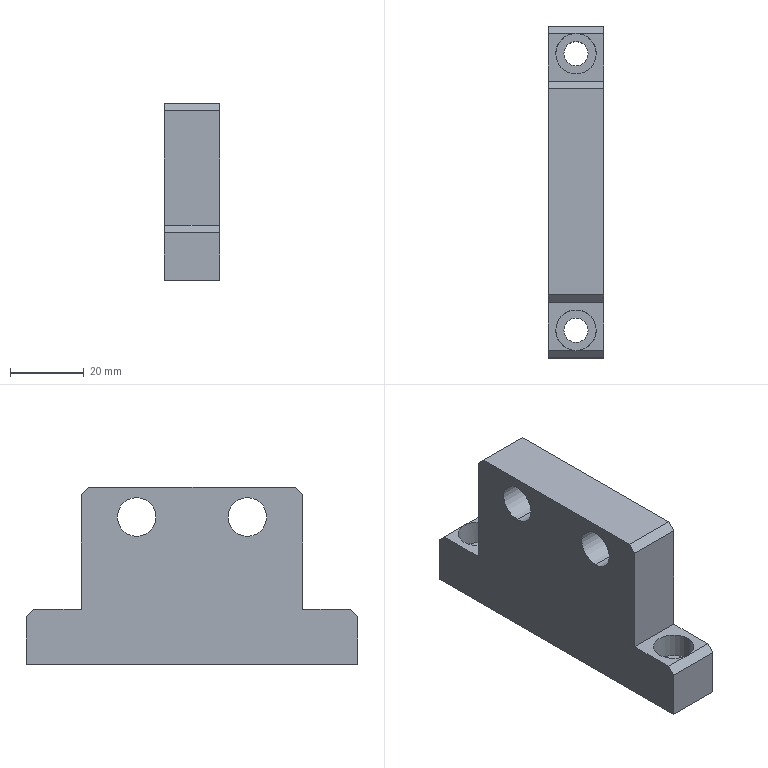Part | SolidWorks | features HoleWzd 2, Chamfer 1, Cut 1, Extrusion 1, MirrorPattern 1 | 1 solid | 28 faces | box 15 x 90 x 48 mm | volume 45379 mm3 | plane 16 | cylinder 12 | commonest cylinder face diameters 6.6 x4 10.5 x4 11 x4
STEP:
#1=CARTESIAN_POINT('',(-7.5,-15.,21.25));
#2=VERTEX_POINT('',#1);
#3=CARTESIAN_POINT('',(-7.5,-15.,10.75));
#4=VERTEX_POINT('',#3);
#5=CARTESIAN_POINT('',(-7.5,-15.,16.));
#6=DIRECTION('',(1.,0.,0.));
#7=DIRECTION('',(0.,0.,-1.));
#8=AXIS2_PLACEMENT_3D('',#5,#6,#7);
#9=CIRCLE('',#8,5.25);
#10=EDGE_CURVE('',#2,#4,#9,.T.);
#11=ORIENTED_EDGE('',*,*,#10,.F.);
#12=CARTESIAN_POINT('',(7.5,-15.,21.25));
#13=VERTEX_POINT('',#12);
#14=CARTESIAN_POINT('',(7.5,-15.,21.25));
#15=DIRECTION('',(1.,0.,0.));
#16=VECTOR('',#15,1000.);
#17=LINE('',#14,#16);
#18=EDGE_CURVE('',#2,#13,#17,.T.);
#19=ORIENTED_EDGE('',*,*,#18,.T.);
#20=CARTESIAN_POINT('',(7.5,-15.,10.75));
#21=VERTEX_POINT('',#20);
#22=CARTESIAN_POINT('',(7.5,-15.,16.));
#23=DIRECTION('',(1.,0.,0.));
#24=DIRECTION('',(0.,0.,-1.));
#25=AXIS2_PLACEMENT_3D('',#22,#23,#24);
#26=CIRCLE('',#25,5.25);
#27=EDGE_CURVE('',#13,#21,#26,.T.);
#28=ORIENTED_EDGE('',*,*,#27,.T.);
#29=CARTESIAN_POINT('',(7.5,-15.,10.75));
#30=DIRECTION('',(1.,0.,0.));
#31=VECTOR('',#30,1000.);
#32=LINE('',#29,#31);
#33=EDGE_CURVE('',#4,#21,#32,.T.);
#34=ORIENTED_EDGE('',*,*,#33,.F.);
#35=EDGE_LOOP('',(#11,#19,#28,#34));
#36=FACE_OUTER_BOUND('',#35,.T.);
#37=CARTESIAN_POINT('',(7.5,-15.,16.));
#38=DIRECTION('',(1.,0.,0.));
#39=DIRECTION('',(0.,0.,-1.));
#40=AXIS2_PLACEMENT_3D('',#37,#38,#39);
#41=CYLINDRICAL_SURFACE('',#40,5.25);
#42=ADVANCED_FACE('',(#36),#41,.F.);
#43=CARTESIAN_POINT('',(-7.5,15.,21.25));
#44=VERTEX_POINT('',#43);
#45=CARTESIAN_POINT('',(-7.5,15.,10.75));
#46=VERTEX_POINT('',#45);
#47=CARTESIAN_POINT('',(-7.5,15.,16.));
#48=DIRECTION('',(1.,0.,0.));
#49=DIRECTION('',(0.,0.,-1.));
#50=AXIS2_PLACEMENT_3D('',#47,#48,#49);
#51=CIRCLE('',#50,5.25);
#52=EDGE_CURVE('',#44,#46,#51,.T.);
#53=ORIENTED_EDGE('',*,*,#52,.F.);
#54=CARTESIAN_POINT('',(7.5,15.,21.25));
#55=VERTEX_POINT('',#54);
#56=CARTESIAN_POINT('',(7.5,15.,21.25));
#57=DIRECTION('',(1.,0.,0.));
#58=VECTOR('',#57,1000.);
#59=LINE('',#56,#58);
#60=EDGE_CURVE('',#44,#55,#59,.T.);
#61=ORIENTED_EDGE('',*,*,#60,.T.);
#62=CARTESIAN_POINT('',(7.5,15.,10.75));
#63=VERTEX_POINT('',#62);
#64=CARTESIAN_POINT('',(7.5,15.,16.));
#65=DIRECTION('',(1.,0.,0.));
#66=DIRECTION('',(0.,0.,-1.));
#67=AXIS2_PLACEMENT_3D('',#64,#65,#66);
#68=CIRCLE('',#67,5.25);
#69=EDGE_CURVE('',#55,#63,#68,.T.);
#70=ORIENTED_EDGE('',*,*,#69,.T.);
#71=CARTESIAN_POINT('',(7.5,15.,10.75));
#72=DIRECTION('',(1.,0.,0.));
#73=VECTOR('',#72,1000.);
#74=LINE('',#71,#73);
#75=EDGE_CURVE('',#46,#63,#74,.T.);
#76=ORIENTED_EDGE('',*,*,#75,.F.);
#77=EDGE_LOOP('',(#53,#61,#70,#76));
#78=FACE_OUTER_BOUND('',#77,.T.);
#79=CARTESIAN_POINT('',(7.5,15.,16.));
#80=DIRECTION('',(1.,0.,0.));
#81=DIRECTION('',(0.,0.,-1.));
#82=AXIS2_PLACEMENT_3D('',#79,#80,#81);
#83=CYLINDRICAL_SURFACE('',#82,5.25);
#84=ADVANCED_FACE('',(#78),#83,.F.);
#85=CARTESIAN_POINT('',(-5.5,-37.5,-15.8));
#86=VERTEX_POINT('',#85);
#87=CARTESIAN_POINT('',(5.5,-37.5,-15.8));
#88=VERTEX_POINT('',#87);
#89=CARTESIAN_POINT('',(0.,-37.5,-15.8));
#90=DIRECTION('',(0.,0.,1.));
#91=DIRECTION('',(1.,0.,0.));
#92=AXIS2_PLACEMENT_3D('',#89,#90,#91);
#93=CIRCLE('',#92,5.5);
#94=EDGE_CURVE('',#86,#88,#93,.T.);
#95=ORIENTED_EDGE('',*,*,#94,.F.);
#96=CARTESIAN_POINT('',(-5.5,-37.5,-9.));
#97=VERTEX_POINT('',#96);
#98=CARTESIAN_POINT('',(-5.5,-37.5,-9.));
#99=DIRECTION('',(0.,0.,1.));
#100=VECTOR('',#99,1000.);
#101=LINE('',#98,#100);
#102=EDGE_CURVE('',#86,#97,#101,.T.);
#103=ORIENTED_EDGE('',*,*,#102,.T.);
#104=CARTESIAN_POINT('',(0.,-43.,-9.));
#105=VERTEX_POINT('',#104);
#106=CARTESIAN_POINT('',(0.,-37.5,-9.));
#107=DIRECTION('',(0.,0.,1.));
#108=DIRECTION('',(1.,0.,0.));
#109=AXIS2_PLACEMENT_3D('',#106,#107,#108);
#110=CIRCLE('',#109,5.5);
#111=EDGE_CURVE('',#97,#105,#110,.T.);
#112=ORIENTED_EDGE('',*,*,#111,.T.);
#113=CARTESIAN_POINT('',(5.5,-37.5,-9.));
#114=VERTEX_POINT('',#113);
#115=CARTESIAN_POINT('',(0.,-37.5,-9.));
#116=DIRECTION('',(0.,0.,1.));
#117=DIRECTION('',(1.,0.,0.));
#118=AXIS2_PLACEMENT_3D('',#115,#116,#117);
#119=CIRCLE('',#118,5.5);
#120=EDGE_CURVE('',#105,#114,#119,.T.);
#121=ORIENTED_EDGE('',*,*,#120,.T.);
#122=CARTESIAN_POINT('',(5.5,-37.5,-9.));
#123=DIRECTION('',(0.,0.,1.));
#124=VECTOR('',#123,1000.);
#125=LINE('',#122,#124);
#126=EDGE_CURVE('',#88,#114,#125,.T.);
#127=ORIENTED_EDGE('',*,*,#126,.F.);
#128=EDGE_LOOP('',(#95,#103,#112,#121,#127));
#129=FACE_OUTER_BOUND('',#128,.T.);
#130=CARTESIAN_POINT('',(0.,-37.5,-9.));
#131=DIRECTION('',(0.,0.,1.));
#132=DIRECTION('',(1.,0.,0.));
#133=AXIS2_PLACEMENT_3D('',#130,#131,#132);
#134=CYLINDRICAL_SURFACE('',#133,5.5);
#135=ADVANCED_FACE('',(#129),#134,.F.);
#136=CARTESIAN_POINT('',(-3.3,-37.5,-24.));
#137=VERTEX_POINT('',#136);
#138=CARTESIAN_POINT('',(3.3,-37.5,-24.));
#139=VERTEX_POINT('',#138);
#140=CARTESIAN_POINT('',(0.,-37.5,-24.));
#141=DIRECTION('',(0.,0.,1.));
#142=DIRECTION('',(1.,0.,0.));
#143=AXIS2_PLACEMENT_3D('',#140,#141,#142);
#144=CIRCLE('',#143,3.3);
#145=EDGE_CURVE('',#137,#139,#144,.T.);
#146=ORIENTED_EDGE('',*,*,#145,.F.);
#147=CARTESIAN_POINT('',(-3.3,-37.5,-15.8));
#148=VERTEX_POINT('',#147);
#149=CARTESIAN_POINT('',(-3.3,-37.5,-9.));
#150=DIRECTION('',(0.,0.,1.));
#151=VECTOR('',#150,1000.);
#152=LINE('',#149,#151);
#153=EDGE_CURVE('',#137,#148,#152,.T.);
#154=ORIENTED_EDGE('',*,*,#153,.T.);
#155=CARTESIAN_POINT('',(3.3,-37.5,-15.8));
#156=VERTEX_POINT('',#155);
#157=CARTESIAN_POINT('',(0.,-37.5,-15.8));
#158=DIRECTION('',(0.,0.,1.));
#159=DIRECTION('',(1.,0.,0.));
#160=AXIS2_PLACEMENT_3D('',#157,#158,#159);
#161=CIRCLE('',#160,3.3);
#162=EDGE_CURVE('',#148,#156,#161,.T.);
#163=ORIENTED_EDGE('',*,*,#162,.T.);
#164=CARTESIAN_POINT('',(3.3,-37.5,-9.));
#165=DIRECTION('',(0.,0.,1.));
#166=VECTOR('',#165,1000.);
#167=LINE('',#164,#166);
#168=EDGE_CURVE('',#139,#156,#167,.T.);
#169=ORIENTED_EDGE('',*,*,#168,.F.);
#170=EDGE_LOOP('',(#146,#154,#163,#169));
#171=FACE_OUTER_BOUND('',#170,.T.);
#172=CARTESIAN_POINT('',(0.,-37.5,-9.));
#173=DIRECTION('',(0.,0.,1.));
#174=DIRECTION('',(1.,0.,0.));
#175=AXIS2_PLACEMENT_3D('',#172,#173,#174);
#176=CYLINDRICAL_SURFACE('',#175,3.3);
#177=ADVANCED_FACE('',(#171),#176,.F.);
#178=CARTESIAN_POINT('',(-5.5,37.5,-15.8));
#179=VERTEX_POINT('',#178);
#180=CARTESIAN_POINT('',(5.5,37.5,-15.8));
#181=VERTEX_POINT('',#180);
#182=CARTESIAN_POINT('',(0.,37.5,-15.8));
#183=DIRECTION('',(0.,0.,1.));
#184=DIRECTION('',(1.,0.,0.));
#185=AXIS2_PLACEMENT_3D('',#182,#183,#184);
#186=CIRCLE('',#185,5.5);
#187=EDGE_CURVE('',#179,#181,#186,.T.);
#188=ORIENTED_EDGE('',*,*,#187,.F.);
#189=CARTESIAN_POINT('',(-5.5,37.5,-9.));
#190=VERTEX_POINT('',#189);
#191=CARTESIAN_POINT('',(-5.5,37.5,-9.));
#192=DIRECTION('',(0.,0.,1.));
#193=VECTOR('',#192,1000.);
#194=LINE('',#191,#193);
#195=EDGE_CURVE('',#179,#190,#194,.T.);
#196=ORIENTED_EDGE('',*,*,#195,.T.);
#197=CARTESIAN_POINT('',(5.5,37.5,-9.));
#198=VERTEX_POINT('',#197);
#199=CARTESIAN_POINT('',(0.,37.5,-9.));
#200=DIRECTION('',(0.,0.,1.));
#201=DIRECTION('',(1.,0.,0.));
#202=AXIS2_PLACEMENT_3D('',#199,#200,#201);
#203=CIRCLE('',#202,5.5);
#204=EDGE_CURVE('',#190,#198,#203,.T.);
#205=ORIENTED_EDGE('',*,*,#204,.T.);
#206=CARTESIAN_POINT('',(5.5,37.5,-9.));
#207=DIRECTION('',(0.,0.,1.));
#208=VECTOR('',#207,1000.);
#209=LINE('',#206,#208);
#210=EDGE_CURVE('',#181,#198,#209,.T.);
#211=ORIENTED_EDGE('',*,*,#210,.F.);
#212=EDGE_LOOP('',(#188,#196,#205,#211));
#213=FACE_OUTER_BOUND('',#212,.T.);
#214=CARTESIAN_POINT('',(0.,37.5,-9.));
#215=DIRECTION('',(0.,0.,1.));
#216=DIRECTION('',(1.,0.,0.));
#217=AXIS2_PLACEMENT_3D('',#214,#215,#216);
#218=CYLINDRICAL_SURFACE('',#217,5.5);
#219=ADVANCED_FACE('',(#213),#218,.F.);
#220=CARTESIAN_POINT('',(-3.3,37.5,-24.));
#221=VERTEX_POINT('',#220);
#222=CARTESIAN_POINT('',(3.3,37.5,-24.));
#223=VERTEX_POINT('',#222);
#224=CARTESIAN_POINT('',(0.,37.5,-24.));
#225=DIRECTION('',(0.,0.,1.));
#226=DIRECTION('',(1.,0.,0.));
#227=AXIS2_PLACEMENT_3D('',#224,#225,#226);
#228=CIRCLE('',#227,3.3);
#229=EDGE_CURVE('',#221,#223,#228,.T.);
#230=ORIENTED_EDGE('',*,*,#229,.F.);
#231=CARTESIAN_POINT('',(-3.3,37.5,-15.8));
#232=VERTEX_POINT('',#231);
#233=CARTESIAN_POINT('',(-3.3,37.5,-9.));
#234=DIRECTION('',(0.,0.,1.));
#235=VECTOR('',#234,1000.);
#236=LINE('',#233,#235);
#237=EDGE_CURVE('',#221,#232,#236,.T.);
#238=ORIENTED_EDGE('',*,*,#237,.T.);
#239=CARTESIAN_POINT('',(3.3,37.5,-15.8));
#240=VERTEX_POINT('',#239);
#241=CARTESIAN_POINT('',(0.,37.5,-15.8));
#242=DIRECTION('',(0.,0.,1.));
#243=DIRECTION('',(1.,0.,0.));
#244=AXIS2_PLACEMENT_3D('',#241,#242,#243);
#245=CIRCLE('',#244,3.3);
#246=EDGE_CURVE('',#232,#240,#245,.T.);
#247=ORIENTED_EDGE('',*,*,#246,.T.);
#248=CARTESIAN_POINT('',(3.3,37.5,-9.));
#249=DIRECTION('',(0.,0.,1.));
#250=VECTOR('',#249,1000.);
#251=LINE('',#248,#250);
#252=EDGE_CURVE('',#223,#240,#251,.T.);
#253=ORIENTED_EDGE('',*,*,#252,.F.);
#254=EDGE_LOOP('',(#230,#238,#247,#253));
#255=FACE_OUTER_BOUND('',#254,.T.);
#256=CARTESIAN_POINT('',(0.,37.5,-9.));
#257=DIRECTION('',(0.,0.,1.));
#258=DIRECTION('',(1.,0.,0.));
#259=AXIS2_PLACEMENT_3D('',#256,#257,#258);
#260=CYLINDRICAL_SURFACE('',#259,3.3);
#261=ADVANCED_FACE('',(#255),#260,.F.);
#262=CARTESIAN_POINT('',(-7.5,-15.,16.));
#263=DIRECTION('',(1.,0.,0.));
#264=DIRECTION('',(0.,0.,-1.));
#265=AXIS2_PLACEMENT_3D('',#262,#263,#264);
#266=CIRCLE('',#265,5.25);
#267=EDGE_CURVE('',#4,#2,#266,.T.);
#268=ORIENTED_EDGE('',*,*,#267,.T.);
#269=ORIENTED_EDGE('',*,*,#10,.T.);
#270=EDGE_LOOP('',(#268,#269));
#271=FACE_BOUND('',#270,.T.);
#272=CARTESIAN_POINT('',(-7.5,15.,16.));
#273=DIRECTION('',(1.,0.,0.));
#274=DIRECTION('',(0.,0.,-1.));
#275=AXIS2_PLACEMENT_3D('',#272,#273,#274);
#276=CIRCLE('',#275,5.25);
#277=EDGE_CURVE('',#46,#44,#276,.T.);
#278=ORIENTED_EDGE('',*,*,#277,.T.);
#279=ORIENTED_EDGE('',*,*,#52,.T.);
#280=EDGE_LOOP('',(#278,#279));
#281=FACE_BOUND('',#280,.T.);
#282=CARTESIAN_POINT('',(-7.5,43.,-9.));
#283=VERTEX_POINT('',#282);
#284=CARTESIAN_POINT('',(-7.5,30.,-9.));
#285=VERTEX_POINT('',#284);
#286=CARTESIAN_POINT('',(-7.5,45.,-9.));
#287=DIRECTION('',(0.,-1.,0.));
#288=VECTOR('',#287,1000.);
#289=LINE('',#286,#288);
#290=EDGE_CURVE('',#283,#285,#289,.T.);
#291=ORIENTED_EDGE('',*,*,#290,.F.);
#292=CARTESIAN_POINT('',(-7.5,45.,-11.));
#293=VERTEX_POINT('',#292);
#294=CARTESIAN_POINT('',(-7.5,45.,-11.));
#295=DIRECTION('',(0.,0.7071,-0.7071));
#296=VECTOR('',#295,1000.);
#297=LINE('',#294,#296);
#298=EDGE_CURVE('',#283,#293,#297,.T.);
#299=ORIENTED_EDGE('',*,*,#298,.T.);
#300=CARTESIAN_POINT('',(-7.5,45.,-24.));
#301=VERTEX_POINT('',#300);
#302=CARTESIAN_POINT('',(-7.5,45.,24.));
#303=DIRECTION('',(0.,0.,1.));
#304=VECTOR('',#303,1000.);
#305=LINE('',#302,#304);
#306=EDGE_CURVE('',#301,#293,#305,.T.);
#307=ORIENTED_EDGE('',*,*,#306,.F.);
#308=CARTESIAN_POINT('',(-7.5,-45.,-24.));
#309=VERTEX_POINT('',#308);
#310=CARTESIAN_POINT('',(-7.5,45.,-24.));
#311=DIRECTION('',(0.,-1.,0.));
#312=VECTOR('',#311,1000.);
#313=LINE('',#310,#312);
#314=EDGE_CURVE('',#301,#309,#313,.T.);
#315=ORIENTED_EDGE('',*,*,#314,.T.);
#316=CARTESIAN_POINT('',(-7.5,-45.,-11.));
#317=VERTEX_POINT('',#316);
#318=CARTESIAN_POINT('',(-7.5,-45.,24.));
#319=DIRECTION('',(0.,0.,1.));
#320=VECTOR('',#319,1000.);
#321=LINE('',#318,#320);
#322=EDGE_CURVE('',#309,#317,#321,.T.);
#323=ORIENTED_EDGE('',*,*,#322,.T.);
#324=CARTESIAN_POINT('',(-7.5,-43.,-9.));
#325=VERTEX_POINT('',#324);
#326=CARTESIAN_POINT('',(-7.5,-43.,-9.));
#327=DIRECTION('',(0.,0.7071,0.7071));
#328=VECTOR('',#327,1000.);
#329=LINE('',#326,#328);
#330=EDGE_CURVE('',#317,#325,#329,.T.);
#331=ORIENTED_EDGE('',*,*,#330,.T.);
#332=CARTESIAN_POINT('',(-7.5,-30.,-9.));
#333=VERTEX_POINT('',#332);
#334=CARTESIAN_POINT('',(-7.5,-45.,-9.));
#335=DIRECTION('',(0.,1.,0.));
#336=VECTOR('',#335,1000.);
#337=LINE('',#334,#336);
#338=EDGE_CURVE('',#325,#333,#337,.T.);
#339=ORIENTED_EDGE('',*,*,#338,.T.);
#340=CARTESIAN_POINT('',(-7.5,-30.,22.));
#341=VERTEX_POINT('',#340);
#342=CARTESIAN_POINT('',(-7.5,-30.,24.));
#343=DIRECTION('',(0.,0.,1.));
#344=VECTOR('',#343,1000.);
#345=LINE('',#342,#344);
#346=EDGE_CURVE('',#333,#341,#345,.T.);
#347=ORIENTED_EDGE('',*,*,#346,.T.);
#348=CARTESIAN_POINT('',(-7.5,-28.,24.));
#349=VERTEX_POINT('',#348);
#350=CARTESIAN_POINT('',(-7.5,-28.,24.));
#351=DIRECTION('',(0.,0.7071,0.7071));
#352=VECTOR('',#351,1000.);
#353=LINE('',#350,#352);
#354=EDGE_CURVE('',#341,#349,#353,.T.);
#355=ORIENTED_EDGE('',*,*,#354,.T.);
#356=CARTESIAN_POINT('',(-7.5,28.,24.));
#357=VERTEX_POINT('',#356);
#358=CARTESIAN_POINT('',(-7.5,45.,24.));
#359=DIRECTION('',(0.,-1.,0.));
#360=VECTOR('',#359,1000.);
#361=LINE('',#358,#360);
#362=EDGE_CURVE('',#357,#349,#361,.T.);
#363=ORIENTED_EDGE('',*,*,#362,.F.);
#364=CARTESIAN_POINT('',(-7.5,30.,22.));
#365=VERTEX_POINT('',#364);
#366=CARTESIAN_POINT('',(-7.5,30.,22.));
#367=DIRECTION('',(0.,0.7071,-0.7071));
#368=VECTOR('',#367,1000.);
#369=LINE('',#366,#368);
#370=EDGE_CURVE('',#357,#365,#369,.T.);
#371=ORIENTED_EDGE('',*,*,#370,.T.);
#372=CARTESIAN_POINT('',(-7.5,30.,24.));
#373=DIRECTION('',(0.,0.,1.));
#374=VECTOR('',#373,1000.);
#375=LINE('',#372,#374);
#376=EDGE_CURVE('',#285,#365,#375,.T.);
#377=ORIENTED_EDGE('',*,*,#376,.F.);
#378=EDGE_LOOP('',(#291,#299,#307,#315,#323,#331,#339,#347,#355,#363,#371,#377));
#379=FACE_OUTER_BOUND('',#378,.T.);
#380=CARTESIAN_POINT('',(-7.5,45.,24.));
#381=DIRECTION('',(1.,0.,0.));
#382=DIRECTION('',(0.,0.,-1.));
#383=AXIS2_PLACEMENT_3D('',#380,#381,#382);
#384=PLANE('',#383);
#385=ADVANCED_FACE('',(#271,#281,#379),#384,.F.);
#386=ORIENTED_EDGE('',*,*,#362,.T.);
#387=CARTESIAN_POINT('',(7.5,-28.,24.));
#388=VERTEX_POINT('',#387);
#389=CARTESIAN_POINT('',(7.5,-28.,24.));
#390=DIRECTION('',(1.,0.,0.));
#391=VECTOR('',#390,1000.);
#392=LINE('',#389,#391);
#393=EDGE_CURVE('',#349,#388,#392,.T.);
#394=ORIENTED_EDGE('',*,*,#393,.T.);
#395=CARTESIAN_POINT('',(7.5,28.,24.));
#396=VERTEX_POINT('',#395);
#397=CARTESIAN_POINT('',(7.5,45.,24.));
#398=DIRECTION('',(0.,-1.,0.));
#399=VECTOR('',#398,1000.);
#400=LINE('',#397,#399);
#401=EDGE_CURVE('',#396,#388,#400,.T.);
#402=ORIENTED_EDGE('',*,*,#401,.F.);
#403=CARTESIAN_POINT('',(-7.5,28.,24.));
#404=DIRECTION('',(-1.,0.,0.));
#405=VECTOR('',#404,1000.);
#406=LINE('',#403,#405);
#407=EDGE_CURVE('',#396,#357,#406,.T.);
#408=ORIENTED_EDGE('',*,*,#407,.T.);
#409=EDGE_LOOP('',(#386,#394,#402,#408));
#410=FACE_OUTER_BOUND('',#409,.T.);
#411=CARTESIAN_POINT('',(7.5,45.,24.));
#412=DIRECTION('',(0.,0.,-1.));
#413=DIRECTION('',(-1.,0.,0.));
#414=AXIS2_PLACEMENT_3D('',#411,#412,#413);
#415=PLANE('',#414);
#416=ADVANCED_FACE('',(#410),#415,.F.);
#417=CARTESIAN_POINT('',(7.5,-15.,16.));
#418=DIRECTION('',(1.,0.,0.));
#419=DIRECTION('',(0.,0.,-1.));
#420=AXIS2_PLACEMENT_3D('',#417,#418,#419);
#421=CIRCLE('',#420,5.25);
#422=EDGE_CURVE('',#21,#13,#421,.T.);
#423=ORIENTED_EDGE('',*,*,#422,.F.);
#424=ORIENTED_EDGE('',*,*,#27,.F.);
#425=EDGE_LOOP('',(#423,#424));
#426=FACE_BOUND('',#425,.T.);
#427=CARTESIAN_POINT('',(7.5,15.,16.));
#428=DIRECTION('',(1.,0.,0.));
#429=DIRECTION('',(0.,0.,-1.));
#430=AXIS2_PLACEMENT_3D('',#427,#428,#429);
#431=CIRCLE('',#430,5.25);
#432=EDGE_CURVE('',#63,#55,#431,.T.);
#433=ORIENTED_EDGE('',*,*,#432,.F.);
#434=ORIENTED_EDGE('',*,*,#69,.F.);
#435=EDGE_LOOP('',(#433,#434));
#436=FACE_BOUND('',#435,.T.);
#437=CARTESIAN_POINT('',(7.5,45.,-11.));
#438=VERTEX_POINT('',#437);
#439=CARTESIAN_POINT('',(7.5,45.,-24.));
#440=VERTEX_POINT('',#439);
#441=CARTESIAN_POINT('',(7.5,45.,24.));
#442=DIRECTION('',(0.,0.,-1.));
#443=VECTOR('',#442,1000.);
#444=LINE('',#441,#443);
#445=EDGE_CURVE('',#438,#440,#444,.T.);
#446=ORIENTED_EDGE('',*,*,#445,.F.);
#447=CARTESIAN_POINT('',(7.5,43.,-9.));
#448=VERTEX_POINT('',#447);
#449=CARTESIAN_POINT('',(7.5,45.,-11.));
#450=DIRECTION('',(0.,-0.7071,0.7071));
#451=VECTOR('',#450,1000.);
#452=LINE('',#449,#451);
#453=EDGE_CURVE('',#438,#448,#452,.T.);
#454=ORIENTED_EDGE('',*,*,#453,.T.);
#455=CARTESIAN_POINT('',(7.5,30.,-9.));
#456=VERTEX_POINT('',#455);
#457=CARTESIAN_POINT('',(7.5,45.,-9.));
#458=DIRECTION('',(0.,-1.,0.));
#459=VECTOR('',#458,1000.);
#460=LINE('',#457,#459);
#461=EDGE_CURVE('',#448,#456,#460,.T.);
#462=ORIENTED_EDGE('',*,*,#461,.T.);
#463=CARTESIAN_POINT('',(7.5,30.,22.));
#464=VERTEX_POINT('',#463);
#465=CARTESIAN_POINT('',(7.5,30.,24.));
#466=DIRECTION('',(0.,0.,1.));
#467=VECTOR('',#466,1000.);
#468=LINE('',#465,#467);
#469=EDGE_CURVE('',#456,#464,#468,.T.);
#470=ORIENTED_EDGE('',*,*,#469,.T.);
#471=CARTESIAN_POINT('',(7.5,30.,22.));
#472=DIRECTION('',(0.,-0.7071,0.7071));
#473=VECTOR('',#472,1000.);
#474=LINE('',#471,#473);
#475=EDGE_CURVE('',#464,#396,#474,.T.);
#476=ORIENTED_EDGE('',*,*,#475,.T.);
#477=ORIENTED_EDGE('',*,*,#401,.T.);
#478=CARTESIAN_POINT('',(7.5,-30.,22.));
#479=VERTEX_POINT('',#478);
#480=CARTESIAN_POINT('',(7.5,-28.,24.));
#481=DIRECTION('',(0.,-0.7071,-0.7071));
#482=VECTOR('',#481,1000.);
#483=LINE('',#480,#482);
#484=EDGE_CURVE('',#388,#479,#483,.T.);
#485=ORIENTED_EDGE('',*,*,#484,.T.);
#486=CARTESIAN_POINT('',(7.5,-30.,-9.));
#487=VERTEX_POINT('',#486);
#488=CARTESIAN_POINT('',(7.5,-30.,24.));
#489=DIRECTION('',(0.,0.,1.));
#490=VECTOR('',#489,1000.);
#491=LINE('',#488,#490);
#492=EDGE_CURVE('',#487,#479,#491,.T.);
#493=ORIENTED_EDGE('',*,*,#492,.F.);
#494=CARTESIAN_POINT('',(7.5,-43.,-9.));
#495=VERTEX_POINT('',#494);
#496=CARTESIAN_POINT('',(7.5,-45.,-9.));
#497=DIRECTION('',(0.,1.,0.));
#498=VECTOR('',#497,1000.);
#499=LINE('',#496,#498);
#500=EDGE_CURVE('',#495,#487,#499,.T.);
#501=ORIENTED_EDGE('',*,*,#500,.F.);
#502=CARTESIAN_POINT('',(7.5,-45.,-11.));
#503=VERTEX_POINT('',#502);
#504=CARTESIAN_POINT('',(7.5,-43.,-9.));
#505=DIRECTION('',(0.,-0.7071,-0.7071));
#506=VECTOR('',#505,1000.);
#507=LINE('',#504,#506);
#508=EDGE_CURVE('',#495,#503,#507,.T.);
#509=ORIENTED_EDGE('',*,*,#508,.T.);
#510=CARTESIAN_POINT('',(7.5,-45.,-24.));
#511=VERTEX_POINT('',#510);
#512=CARTESIAN_POINT('',(7.5,-45.,24.));
#513=DIRECTION('',(0.,0.,-1.));
#514=VECTOR('',#513,1000.);
#515=LINE('',#512,#514);
#516=EDGE_CURVE('',#503,#511,#515,.T.);
#517=ORIENTED_EDGE('',*,*,#516,.T.);
#518=CARTESIAN_POINT('',(7.5,45.,-24.));
#519=DIRECTION('',(0.,-1.,0.));
#520=VECTOR('',#519,1000.);
#521=LINE('',#518,#520);
#522=EDGE_CURVE('',#440,#511,#521,.T.);
#523=ORIENTED_EDGE('',*,*,#522,.F.);
#524=EDGE_LOOP('',(#446,#454,#462,#470,#476,#477,#485,#493,#501,#509,#517,#523));
#525=FACE_OUTER_BOUND('',#524,.T.);
#526=CARTESIAN_POINT('',(7.5,45.,24.));
#527=DIRECTION('',(-1.,0.,0.));
#528=DIRECTION('',(0.,0.,1.));
#529=AXIS2_PLACEMENT_3D('',#526,#527,#528);
#530=PLANE('',#529);
#531=ADVANCED_FACE('',(#426,#436,#525),#530,.F.);
#532=ORIENTED_EDGE('',*,*,#306,.T.);
#533=CARTESIAN_POINT('',(0.,45.,-11.));
#534=DIRECTION('',(1.,0.,0.));
#535=VECTOR('',#534,1000.);
#536=LINE('',#533,#535);
#537=EDGE_CURVE('',#293,#438,#536,.T.);
#538=ORIENTED_EDGE('',*,*,#537,.T.);
#539=ORIENTED_EDGE('',*,*,#445,.T.);
#540=CARTESIAN_POINT('',(7.5,45.,-24.));
#541=DIRECTION('',(-1.,0.,0.));
#542=VECTOR('',#541,1000.);
#543=LINE('',#540,#542);
#544=EDGE_CURVE('',#440,#301,#543,.T.);
#545=ORIENTED_EDGE('',*,*,#544,.T.);
#546=EDGE_LOOP('',(#532,#538,#539,#545));
#547=FACE_OUTER_BOUND('',#546,.T.);
#548=CARTESIAN_POINT('',(0.,45.,0.));
#549=DIRECTION('',(0.,1.,0.));
#550=DIRECTION('',(0.,0.,1.));
#551=AXIS2_PLACEMENT_3D('',#548,#549,#550);
#552=PLANE('',#551);
#553=ADVANCED_FACE('',(#547),#552,.T.);
#554=CARTESIAN_POINT('',(0.,-37.5,-24.));
#555=DIRECTION('',(0.,0.,1.));
#556=DIRECTION('',(1.,0.,0.));
#557=AXIS2_PLACEMENT_3D('',#554,#555,#556);
#558=CIRCLE('',#557,3.3);
#559=EDGE_CURVE('',#139,#137,#558,.T.);
#560=ORIENTED_EDGE('',*,*,#559,.T.);
#561=ORIENTED_EDGE('',*,*,#145,.T.);
#562=EDGE_LOOP('',(#560,#561));
#563=FACE_BOUND('',#562,.T.);
#564=CARTESIAN_POINT('',(0.,37.5,-24.));
#565=DIRECTION('',(0.,0.,1.));
#566=DIRECTION('',(1.,0.,0.));
#567=AXIS2_PLACEMENT_3D('',#564,#565,#566);
#568=CIRCLE('',#567,3.3);
#569=EDGE_CURVE('',#223,#221,#568,.T.);
#570=ORIENTED_EDGE('',*,*,#569,.T.);
#571=ORIENTED_EDGE('',*,*,#229,.T.);
#572=EDGE_LOOP('',(#570,#571));
#573=FACE_BOUND('',#572,.T.);
#574=CARTESIAN_POINT('',(7.5,-45.,-24.));
#575=DIRECTION('',(-1.,0.,0.));
#576=VECTOR('',#575,1000.);
#577=LINE('',#574,#576);
#578=EDGE_CURVE('',#511,#309,#577,.T.);
#579=ORIENTED_EDGE('',*,*,#578,.T.);
#580=ORIENTED_EDGE('',*,*,#314,.F.);
#581=ORIENTED_EDGE('',*,*,#544,.F.);
#582=ORIENTED_EDGE('',*,*,#522,.T.);
#583=EDGE_LOOP('',(#579,#580,#581,#582));
#584=FACE_OUTER_BOUND('',#583,.T.);
#585=CARTESIAN_POINT('',(7.5,45.,-24.));
#586=DIRECTION('',(0.,0.,1.));
#587=DIRECTION('',(1.,0.,0.));
#588=AXIS2_PLACEMENT_3D('',#585,#586,#587);
#589=PLANE('',#588);
#590=ADVANCED_FACE('',(#563,#573,#584),#589,.F.);
#591=ORIENTED_EDGE('',*,*,#516,.F.);
#592=CARTESIAN_POINT('',(0.,-45.,-11.));
#593=DIRECTION('',(-1.,0.,0.));
#594=VECTOR('',#593,1000.);
#595=LINE('',#592,#594);
#596=EDGE_CURVE('',#503,#317,#595,.T.);
#597=ORIENTED_EDGE('',*,*,#596,.T.);
#598=ORIENTED_EDGE('',*,*,#322,.F.);
#599=ORIENTED_EDGE('',*,*,#578,.F.);
#600=EDGE_LOOP('',(#591,#597,#598,#599));
#601=FACE_OUTER_BOUND('',#600,.T.);
#602=CARTESIAN_POINT('',(0.,-45.,0.));
#603=DIRECTION('',(0.,1.,0.));
#604=DIRECTION('',(0.,0.,1.));
#605=AXIS2_PLACEMENT_3D('',#602,#603,#604);
#606=PLANE('',#605);
#607=ADVANCED_FACE('',(#601),#606,.F.);
#608=ORIENTED_EDGE('',*,*,#492,.T.);
#609=CARTESIAN_POINT('',(-7.5,-30.,22.));
#610=DIRECTION('',(-1.,0.,0.));
#611=VECTOR('',#610,1000.);
#612=LINE('',#609,#611);
#613=EDGE_CURVE('',#479,#341,#612,.T.);
#614=ORIENTED_EDGE('',*,*,#613,.T.);
#615=ORIENTED_EDGE('',*,*,#346,.F.);
#616=CARTESIAN_POINT('',(-7.5,-30.,-9.));
#617=DIRECTION('',(1.,0.,0.));
#618=VECTOR('',#617,1000.);
#619=LINE('',#616,#618);
#620=EDGE_CURVE('',#333,#487,#619,.T.);
#621=ORIENTED_EDGE('',*,*,#620,.T.);
#622=EDGE_LOOP('',(#608,#614,#615,#621));
#623=FACE_OUTER_BOUND('',#622,.T.);
#624=CARTESIAN_POINT('',(-7.5,-30.,24.));
#625=DIRECTION('',(0.,1.,0.));
#626=DIRECTION('',(0.,0.,1.));
#627=AXIS2_PLACEMENT_3D('',#624,#625,#626);
#628=PLANE('',#627);
#629=ADVANCED_FACE('',(#623),#628,.F.);
#630=ORIENTED_EDGE('',*,*,#338,.F.);
#631=CARTESIAN_POINT('',(-7.5,-43.,-9.));
#632=DIRECTION('',(1.,0.,0.));
#633=VECTOR('',#632,1000.);
#634=LINE('',#631,#633);
#635=EDGE_CURVE('',#325,#105,#634,.T.);
#636=ORIENTED_EDGE('',*,*,#635,.T.);
#637=ORIENTED_EDGE('',*,*,#111,.F.);
#638=CARTESIAN_POINT('',(0.,-37.5,-9.));
#639=DIRECTION('',(0.,0.,1.));
#640=DIRECTION('',(1.,0.,0.));
#641=AXIS2_PLACEMENT_3D('',#638,#639,#640);
#642=CIRCLE('',#641,5.5);
#643=EDGE_CURVE('',#114,#97,#642,.T.);
#644=ORIENTED_EDGE('',*,*,#643,.F.);
#645=ORIENTED_EDGE('',*,*,#120,.F.);
#646=CARTESIAN_POINT('',(-7.5,-43.,-9.));
#647=DIRECTION('',(1.,0.,0.));
#648=VECTOR('',#647,1000.);
#649=LINE('',#646,#648);
#650=EDGE_CURVE('',#105,#495,#649,.T.);
#651=ORIENTED_EDGE('',*,*,#650,.T.);
#652=ORIENTED_EDGE('',*,*,#500,.T.);
#653=ORIENTED_EDGE('',*,*,#620,.F.);
#654=EDGE_LOOP('',(#630,#636,#637,#644,#645,#651,#652,#653));
#655=FACE_OUTER_BOUND('',#654,.T.);
#656=CARTESIAN_POINT('',(-7.5,-45.,-9.));
#657=DIRECTION('',(0.,0.,-1.));
#658=DIRECTION('',(-1.,0.,0.));
#659=AXIS2_PLACEMENT_3D('',#656,#657,#658);
#660=PLANE('',#659);
#661=ADVANCED_FACE('',(#655),#660,.F.);
#662=ORIENTED_EDGE('',*,*,#461,.F.);
#663=CARTESIAN_POINT('',(0.,43.,-9.));
#664=VERTEX_POINT('',#663);
#665=CARTESIAN_POINT('',(-7.5,43.,-9.));
#666=DIRECTION('',(-1.,0.,0.));
#667=VECTOR('',#666,1000.);
#668=LINE('',#665,#667);
#669=EDGE_CURVE('',#448,#664,#668,.T.);
#670=ORIENTED_EDGE('',*,*,#669,.T.);
#671=CARTESIAN_POINT('',(0.,37.5,-9.));
#672=DIRECTION('',(0.,0.,1.));
#673=DIRECTION('',(1.,0.,0.));
#674=AXIS2_PLACEMENT_3D('',#671,#672,#673);
#675=CIRCLE('',#674,5.5);
#676=EDGE_CURVE('',#198,#664,#675,.T.);
#677=ORIENTED_EDGE('',*,*,#676,.F.);
#678=ORIENTED_EDGE('',*,*,#204,.F.);
#679=CARTESIAN_POINT('',(0.,37.5,-9.));
#680=DIRECTION('',(0.,0.,1.));
#681=DIRECTION('',(1.,0.,0.));
#682=AXIS2_PLACEMENT_3D('',#679,#680,#681);
#683=CIRCLE('',#682,5.5);
#684=EDGE_CURVE('',#664,#190,#683,.T.);
#685=ORIENTED_EDGE('',*,*,#684,.F.);
#686=CARTESIAN_POINT('',(-7.5,43.,-9.));
#687=DIRECTION('',(-1.,0.,0.));
#688=VECTOR('',#687,1000.);
#689=LINE('',#686,#688);
#690=EDGE_CURVE('',#664,#283,#689,.T.);
#691=ORIENTED_EDGE('',*,*,#690,.T.);
#692=ORIENTED_EDGE('',*,*,#290,.T.);
#693=CARTESIAN_POINT('',(-7.5,30.,-9.));
#694=DIRECTION('',(1.,0.,0.));
#695=VECTOR('',#694,1000.);
#696=LINE('',#693,#695);
#697=EDGE_CURVE('',#285,#456,#696,.T.);
#698=ORIENTED_EDGE('',*,*,#697,.T.);
#699=EDGE_LOOP('',(#662,#670,#677,#678,#685,#691,#692,#698));
#700=FACE_OUTER_BOUND('',#699,.T.);
#701=CARTESIAN_POINT('',(-7.5,45.,-9.));
#702=DIRECTION('',(0.,0.,1.));
#703=DIRECTION('',(1.,0.,0.));
#704=AXIS2_PLACEMENT_3D('',#701,#702,#703);
#705=PLANE('',#704);
#706=ADVANCED_FACE('',(#700),#705,.T.);
#707=ORIENTED_EDGE('',*,*,#376,.T.);
#708=CARTESIAN_POINT('',(7.5,30.,22.));
#709=DIRECTION('',(1.,0.,0.));
#710=VECTOR('',#709,1000.);
#711=LINE('',#708,#710);
#712=EDGE_CURVE('',#365,#464,#711,.T.);
#713=ORIENTED_EDGE('',*,*,#712,.T.);
#714=ORIENTED_EDGE('',*,*,#469,.F.);
#715=ORIENTED_EDGE('',*,*,#697,.F.);
#716=EDGE_LOOP('',(#707,#713,#714,#715));
#717=FACE_OUTER_BOUND('',#716,.T.);
#718=CARTESIAN_POINT('',(-7.5,30.,24.));
#719=DIRECTION('',(0.,1.,0.));
#720=DIRECTION('',(0.,0.,1.));
#721=AXIS2_PLACEMENT_3D('',#718,#719,#720);
#722=PLANE('',#721);
#723=ADVANCED_FACE('',(#717),#722,.T.);
#724=ORIENTED_EDGE('',*,*,#237,.F.);
#725=ORIENTED_EDGE('',*,*,#569,.F.);
#726=ORIENTED_EDGE('',*,*,#252,.T.);
#727=CARTESIAN_POINT('',(0.,37.5,-15.8));
#728=DIRECTION('',(0.,0.,1.));
#729=DIRECTION('',(1.,0.,0.));
#730=AXIS2_PLACEMENT_3D('',#727,#728,#729);
#731=CIRCLE('',#730,3.3);
#732=EDGE_CURVE('',#240,#232,#731,.T.);
#733=ORIENTED_EDGE('',*,*,#732,.T.);
#734=EDGE_LOOP('',(#724,#725,#726,#733));
#735=FACE_OUTER_BOUND('',#734,.T.);
#736=CARTESIAN_POINT('',(0.,37.5,-9.));
#737=DIRECTION('',(0.,0.,1.));
#738=DIRECTION('',(1.,0.,0.));
#739=AXIS2_PLACEMENT_3D('',#736,#737,#738);
#740=CYLINDRICAL_SURFACE('',#739,3.3);
#741=ADVANCED_FACE('',(#735),#740,.F.);
#742=ORIENTED_EDGE('',*,*,#732,.F.);
#743=ORIENTED_EDGE('',*,*,#246,.F.);
#744=EDGE_LOOP('',(#742,#743));
#745=FACE_BOUND('',#744,.T.);
#746=CARTESIAN_POINT('',(0.,37.5,-15.8));
#747=DIRECTION('',(0.,0.,1.));
#748=DIRECTION('',(1.,0.,0.));
#749=AXIS2_PLACEMENT_3D('',#746,#747,#748);
#750=CIRCLE('',#749,5.5);
#751=EDGE_CURVE('',#181,#179,#750,.T.);
#752=ORIENTED_EDGE('',*,*,#751,.T.);
#753=ORIENTED_EDGE('',*,*,#187,.T.);
#754=EDGE_LOOP('',(#752,#753));
#755=FACE_OUTER_BOUND('',#754,.T.);
#756=CARTESIAN_POINT('',(3.3,37.5,-15.8));
#757=DIRECTION('',(0.,0.,-1.));
#758=DIRECTION('',(-1.,0.,0.));
#759=AXIS2_PLACEMENT_3D('',#756,#757,#758);
#760=PLANE('',#759);
#761=ADVANCED_FACE('',(#745,#755),#760,.F.);
#762=ORIENTED_EDGE('',*,*,#195,.F.);
#763=ORIENTED_EDGE('',*,*,#751,.F.);
#764=ORIENTED_EDGE('',*,*,#210,.T.);
#765=ORIENTED_EDGE('',*,*,#676,.T.);
#766=ORIENTED_EDGE('',*,*,#684,.T.);
#767=EDGE_LOOP('',(#762,#763,#764,#765,#766));
#768=FACE_OUTER_BOUND('',#767,.T.);
#769=CARTESIAN_POINT('',(0.,37.5,-9.));
#770=DIRECTION('',(0.,0.,1.));
#771=DIRECTION('',(1.,0.,0.));
#772=AXIS2_PLACEMENT_3D('',#769,#770,#771);
#773=CYLINDRICAL_SURFACE('',#772,5.5);
#774=ADVANCED_FACE('',(#768),#773,.F.);
#775=ORIENTED_EDGE('',*,*,#153,.F.);
#776=ORIENTED_EDGE('',*,*,#559,.F.);
#777=ORIENTED_EDGE('',*,*,#168,.T.);
#778=CARTESIAN_POINT('',(0.,-37.5,-15.8));
#779=DIRECTION('',(0.,0.,1.));
#780=DIRECTION('',(1.,0.,0.));
#781=AXIS2_PLACEMENT_3D('',#778,#779,#780);
#782=CIRCLE('',#781,3.3);
#783=EDGE_CURVE('',#156,#148,#782,.T.);
#784=ORIENTED_EDGE('',*,*,#783,.T.);
#785=EDGE_LOOP('',(#775,#776,#777,#784));
#786=FACE_OUTER_BOUND('',#785,.T.);
#787=CARTESIAN_POINT('',(0.,-37.5,-9.));
#788=DIRECTION('',(0.,0.,1.));
#789=DIRECTION('',(1.,0.,0.));
#790=AXIS2_PLACEMENT_3D('',#787,#788,#789);
#791=CYLINDRICAL_SURFACE('',#790,3.3);
#792=ADVANCED_FACE('',(#786),#791,.F.);
#793=ORIENTED_EDGE('',*,*,#783,.F.);
#794=ORIENTED_EDGE('',*,*,#162,.F.);
#795=EDGE_LOOP('',(#793,#794));
#796=FACE_BOUND('',#795,.T.);
#797=CARTESIAN_POINT('',(0.,-37.5,-15.8));
#798=DIRECTION('',(0.,0.,1.));
#799=DIRECTION('',(1.,0.,0.));
#800=AXIS2_PLACEMENT_3D('',#797,#798,#799);
#801=CIRCLE('',#800,5.5);
#802=EDGE_CURVE('',#88,#86,#801,.T.);
#803=ORIENTED_EDGE('',*,*,#802,.T.);
#804=ORIENTED_EDGE('',*,*,#94,.T.);
#805=EDGE_LOOP('',(#803,#804));
#806=FACE_OUTER_BOUND('',#805,.T.);
#807=CARTESIAN_POINT('',(3.3,-37.5,-15.8));
#808=DIRECTION('',(0.,0.,-1.));
#809=DIRECTION('',(-1.,0.,0.));
#810=AXIS2_PLACEMENT_3D('',#807,#808,#809);
#811=PLANE('',#810);
#812=ADVANCED_FACE('',(#796,#806),#811,.F.);
#813=ORIENTED_EDGE('',*,*,#102,.F.);
#814=ORIENTED_EDGE('',*,*,#802,.F.);
#815=ORIENTED_EDGE('',*,*,#126,.T.);
#816=ORIENTED_EDGE('',*,*,#643,.T.);
#817=EDGE_LOOP('',(#813,#814,#815,#816));
#818=FACE_OUTER_BOUND('',#817,.T.);
#819=CARTESIAN_POINT('',(0.,-37.5,-9.));
#820=DIRECTION('',(0.,0.,1.));
#821=DIRECTION('',(1.,0.,0.));
#822=AXIS2_PLACEMENT_3D('',#819,#820,#821);
#823=CYLINDRICAL_SURFACE('',#822,5.5);
#824=ADVANCED_FACE('',(#818),#823,.F.);
#825=ORIENTED_EDGE('',*,*,#60,.F.);
#826=ORIENTED_EDGE('',*,*,#277,.F.);
#827=ORIENTED_EDGE('',*,*,#75,.T.);
#828=ORIENTED_EDGE('',*,*,#432,.T.);
#829=EDGE_LOOP('',(#825,#826,#827,#828));
#830=FACE_OUTER_BOUND('',#829,.T.);
#831=CARTESIAN_POINT('',(7.5,15.,16.));
#832=DIRECTION('',(1.,0.,0.));
#833=DIRECTION('',(0.,0.,-1.));
#834=AXIS2_PLACEMENT_3D('',#831,#832,#833);
#835=CYLINDRICAL_SURFACE('',#834,5.25);
#836=ADVANCED_FACE('',(#830),#835,.F.);
#837=ORIENTED_EDGE('',*,*,#18,.F.);
#838=ORIENTED_EDGE('',*,*,#267,.F.);
#839=ORIENTED_EDGE('',*,*,#33,.T.);
#840=ORIENTED_EDGE('',*,*,#422,.T.);
#841=EDGE_LOOP('',(#837,#838,#839,#840));
#842=FACE_OUTER_BOUND('',#841,.T.);
#843=CARTESIAN_POINT('',(7.5,-15.,16.));
#844=DIRECTION('',(1.,0.,0.));
#845=DIRECTION('',(0.,0.,-1.));
#846=AXIS2_PLACEMENT_3D('',#843,#844,#845);
#847=CYLINDRICAL_SURFACE('',#846,5.25);
#848=ADVANCED_FACE('',(#842),#847,.F.);
#849=ORIENTED_EDGE('',*,*,#690,.F.);
#850=ORIENTED_EDGE('',*,*,#669,.F.);
#851=ORIENTED_EDGE('',*,*,#453,.F.);
#852=ORIENTED_EDGE('',*,*,#537,.F.);
#853=ORIENTED_EDGE('',*,*,#298,.F.);
#854=EDGE_LOOP('',(#849,#850,#851,#852,#853));
#855=FACE_OUTER_BOUND('',#854,.T.);
#856=CARTESIAN_POINT('',(0.,45.,-11.));
#857=DIRECTION('',(0.,-0.7071,-0.7071));
#858=DIRECTION('',(1.,0.,0.));
#859=AXIS2_PLACEMENT_3D('',#856,#857,#858);
#860=PLANE('',#859);
#861=ADVANCED_FACE('',(#855),#860,.F.);
#862=ORIENTED_EDGE('',*,*,#330,.F.);
#863=ORIENTED_EDGE('',*,*,#596,.F.);
#864=ORIENTED_EDGE('',*,*,#508,.F.);
#865=ORIENTED_EDGE('',*,*,#650,.F.);
#866=ORIENTED_EDGE('',*,*,#635,.F.);
#867=EDGE_LOOP('',(#862,#863,#864,#865,#866));
#868=FACE_OUTER_BOUND('',#867,.T.);
#869=CARTESIAN_POINT('',(-7.5,-43.,-9.));
#870=DIRECTION('',(0.,0.7071,-0.7071));
#871=DIRECTION('',(1.,0.,0.));
#872=AXIS2_PLACEMENT_3D('',#869,#870,#871);
#873=PLANE('',#872);
#874=ADVANCED_FACE('',(#868),#873,.F.);
#875=ORIENTED_EDGE('',*,*,#354,.F.);
#876=ORIENTED_EDGE('',*,*,#613,.F.);
#877=ORIENTED_EDGE('',*,*,#484,.F.);
#878=ORIENTED_EDGE('',*,*,#393,.F.);
#879=EDGE_LOOP('',(#875,#876,#877,#878));
#880=FACE_OUTER_BOUND('',#879,.T.);
#881=CARTESIAN_POINT('',(7.5,-28.,24.));
#882=DIRECTION('',(0.,0.7071,-0.7071));
#883=DIRECTION('',(1.,0.,0.));
#884=AXIS2_PLACEMENT_3D('',#881,#882,#883);
#885=PLANE('',#884);
#886=ADVANCED_FACE('',(#880),#885,.F.);
#887=ORIENTED_EDGE('',*,*,#370,.F.);
#888=ORIENTED_EDGE('',*,*,#407,.F.);
#889=ORIENTED_EDGE('',*,*,#475,.F.);
#890=ORIENTED_EDGE('',*,*,#712,.F.);
#891=EDGE_LOOP('',(#887,#888,#889,#890));
#892=FACE_OUTER_BOUND('',#891,.T.);
#893=CARTESIAN_POINT('',(-7.5,30.,22.));
#894=DIRECTION('',(0.,0.7071,0.7071));
#895=DIRECTION('',(-1.,0.,0.));
#896=AXIS2_PLACEMENT_3D('',#893,#894,#895);
#897=PLANE('',#896);
#898=ADVANCED_FACE('',(#892),#897,.T.);
#899=CLOSED_SHELL('',(#42,#84,#135,#177,#219,#261,#385,#416,#531,#553,#590,#607,#629,#661,#706,#723,#741,#761,#774,#792,#812,#824,#836,#848,#861,#874,#886,#898));
#900=MANIFOLD_SOLID_BREP('',#899);
#901=CARTESIAN_POINT('',(0.,0.,0.));
#902=DIRECTION('',(0.,0.,1.));
#903=DIRECTION('',(1.,0.,0.));
#904=AXIS2_PLACEMENT_3D('',#901,#902,#903);
#905=(LENGTH_UNIT()NAMED_UNIT(*)SI_UNIT(.MILLI.,.METRE.));
#906=UNCERTAINTY_MEASURE_WITH_UNIT(LENGTH_MEASURE(0.00001),#905,'','');
#907=(NAMED_UNIT(*)PLANE_ANGLE_UNIT()SI_UNIT($,.RADIAN.));
#908=(NAMED_UNIT(*)SI_UNIT($,.STERADIAN.)SOLID_ANGLE_UNIT());
#909=(GEOMETRIC_REPRESENTATION_CONTEXT(3)GLOBAL_UNCERTAINTY_ASSIGNED_CONTEXT((#906))GLOBAL_UNIT_ASSIGNED_CONTEXT((#905,#907,#908))REPRESENTATION_CONTEXT('',''));
#910=ADVANCED_BREP_SHAPE_REPRESENTATION('',(#900,#904),#909);